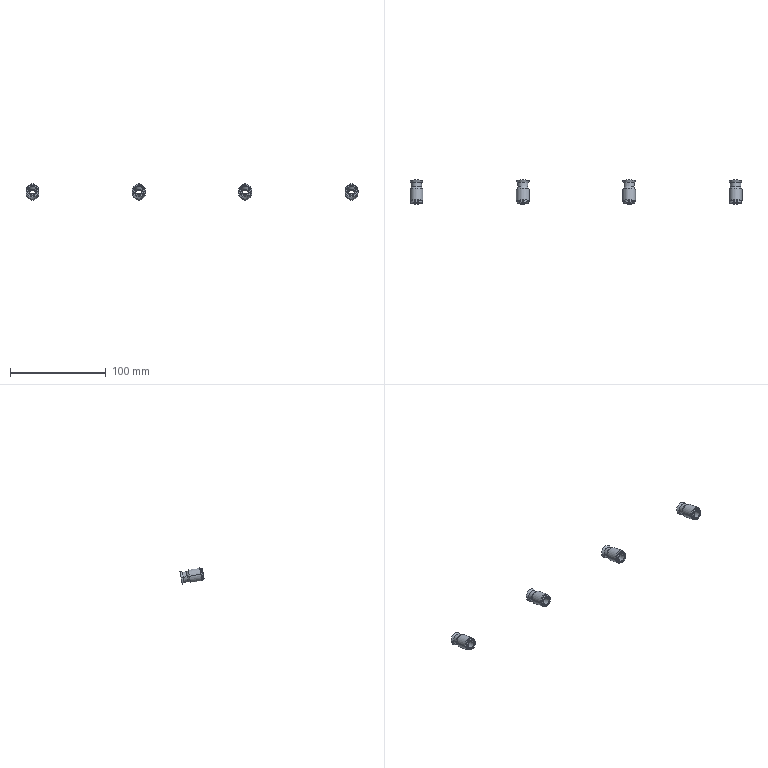Part | SolidWorks | 4 solids | 112 faces | box 346.5 x 25.199 x 16.948 mm | volume 7226 mm3 | cylinder 56 | plane 24 | cone 24 | torus 8 | commonest cylinder face diameters 8 x16 6.476 x8 10.8 x8 10.935 x8 12.15 x8 13.5 x8